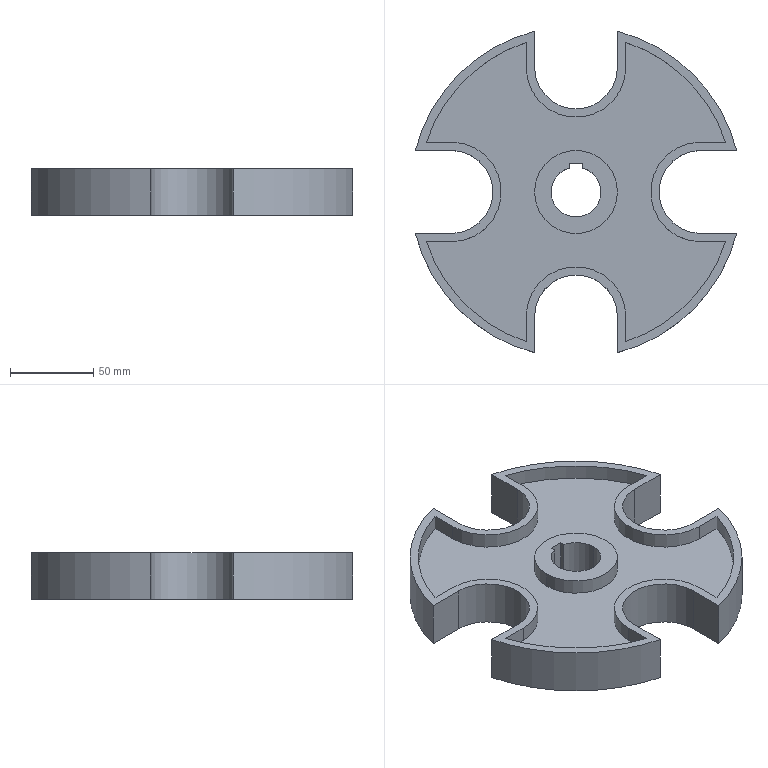Part | SolidWorks | features BaseBody 1 | 1 solid | 64 faces | box 193.649 x 193.649 x 28 mm | volume 321506 mm3 | plane 33 | cylinder 31 | commonest cylinder face diameters 50 x8 60 x8 190 x8 200 x4 30 x3